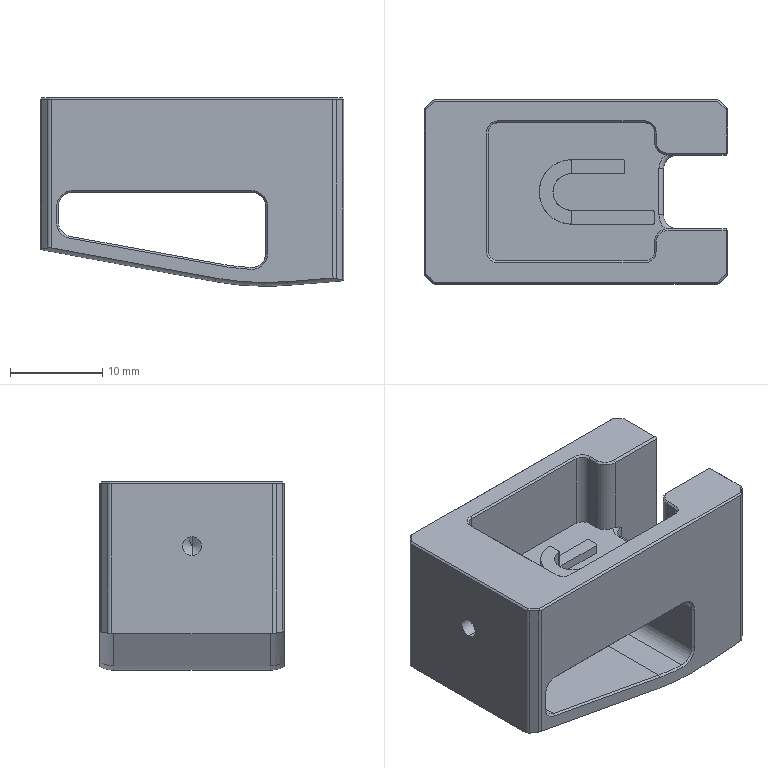NC program | NX | posted with a generic post | part box 33 x 20 x 20.478 mm
Lines 3414 to 3438 of 3438:
(PLANAR_MILL_COPY_COPY_COPY_COPY_COPY_COPY_1_COPY , TOOL : D6A45)
N6814 T01 M6
N6816 G54
N6818 G17 G0 G90 X-15.413 Y4.109 B0. C0. S9500 M3
N6820 G43 Z30. H1
N6822 Z0.5
N6824 G94 G1 Z-1. F1250.
N6826 G3 X-16.061 Y3.347 R1.
N6828 G1 X-17.231 Y-3.028
N6830 G3 X-17.638 Y-6.462 R27.2
N6832 X-16.939 Y-7.2 R0.7
N6834 G1 X-11.8
N6836 G3 X-11.1 Y-6.5 R0.7
N6838 G1 Y13.
N6840 G3 X-11.8 Y13.7 R0.7
N6842 G1 X-13.577
N6844 G3 X-14.266 Y13.126 R0.7
N6846 G1 X-16.061 Y3.347
N6848 G3 X-15.726 Y2.405 R1.
N6850 G1 Z0.5
N6852 G0 Z30.
N6854 M5
N6856 M2